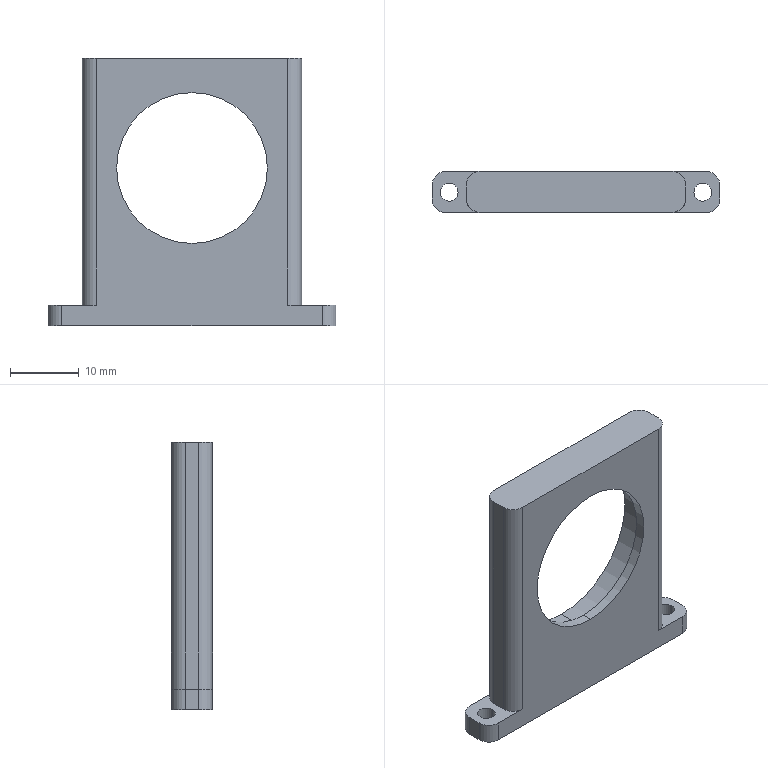NC program | NX | posted with a generic post | part box 42 x 6 x 39 mm
Whole program:
N10 G17 G21 G94 G90
(HOLE_MILLING , TOOL : D10JING)
N12 T14 M6
N14 G54
N16 G17 G0 G90 X0. Y-3.5 B0. C0. S9500 M3
N18 G43 Z30. H14
N20 Z0.5
N22 G94 G3 X2.025 Y-5.525 R2.025 F1250.
N24 X4.05 Y-3.5 R2.025
N26 X4.05 Y-3.5 Z-0.3 I-4.05 J0.
N28 X4.05 Y-3.5 Z-1.1 I-4.05 J0.
N30 X4.05 Y-3.5 Z-1.9 I-4.05 J0.
N32 X4.05 Y-3.5 Z-2.7 I-4.05 J0.
N34 X4.05 Y-3.5 Z-3.5 I-4.05 J0.
N36 X4.05 Y-3.5 Z-4.3 I-4.05 J0.
N38 X0. Y0.55 Z-4.5 R4.05
N40 X-4.05 Y-3.5 R4.05
N42 X0. Y0.55 R-4.05
N44 X-2.025 Y-1.475 R2.025
N46 X0. Y-3.5 R2.025
N48 G0 Z0.5
N50 G3 X4.05 Y-7.55 R4.05
N52 X8.1 Y-3.5 R4.05
N54 X8.1 Y-3.5 Z-0.3 I-8.1 J0.
N56 X8.1 Y-3.5 Z-1.1 I-8.1 J0.
N58 X8.1 Y-3.5 Z-1.9 I-8.1 J0.
N60 X8.1 Y-3.5 Z-2.7 I-8.1 J0.
N62 X8.1 Y-3.5 Z-3.5 I-8.1 J0.
N64 X8.1 Y-3.5 Z-4.3 I-8.1 J0.
N66 X0. Y4.6 Z-4.5 R8.1
N68 X-8.1 Y-3.5 R8.1
N70 X0. Y4.6 R-8.1
N72 X-4.05 Y0.55 R4.05
N74 X0. Y-3.5 R4.05
N76 G0 Z30.
(HOLE_MILLING_COPY , TOOL : D10JING)
N78 Z-4.
N80 G3 X1.5 Y-5. R1.5
N82 X3. Y-3.5 R1.5
N84 X3. Y-3.5 Z-4.8 I-3. J0.
N86 X3. Y-3.5 Z-5.6 I-3. J0.
N88 X-3. Y-3.5 Z-6. I-3. J0.
N90 X0. Y-6.5 R3.
N92 X-3. Y-3.5 R-3.
N94 X-1.5 Y-5. R1.5
N96 X0. Y-3.5 R1.5
N98 G0 Z-4.
N100 G3 X3. Y-6.5 R3.
N102 X6. Y-3.5 R3.
N104 X6. Y-3.5 Z-4.8 I-6. J0.
N106 X6. Y-3.5 Z-5.6 I-6. J0.
N108 X-6. Y-3.5 Z-6. I-6. J0.
N110 X0. Y-9.5 R6.
N112 X-6. Y-3.5 R-6.
N114 X-3. Y-6.5 R3.
N116 X0. Y-3.5 R3.
N118 G0 Z30.
N120 M5
(PLANAR_MILL_COPY_COPY_COPY_COPY_COPY_COPY_1_COPY_1_COPY_COPY , TOOL : D6A45)
N122 T01 M6
N124 G54
N126 G17 G0 G90 X-0.866 Y-15.3 B0. C0. S9500 M3
N128 G43 Z30. H1
N130 Z0.5
N132 G94 G1 Z-1. F1250.
N134 G3 X0. Y-15.8 R1.
N136 X12.3 Y-3.5 R12.3
N138 X0. Y-15.8 R-12.3
N140 X0.866 Y-15.3 R1.
N142 G1 Z0.5
N144 G0 Z30.
N146 M5
N148 M2